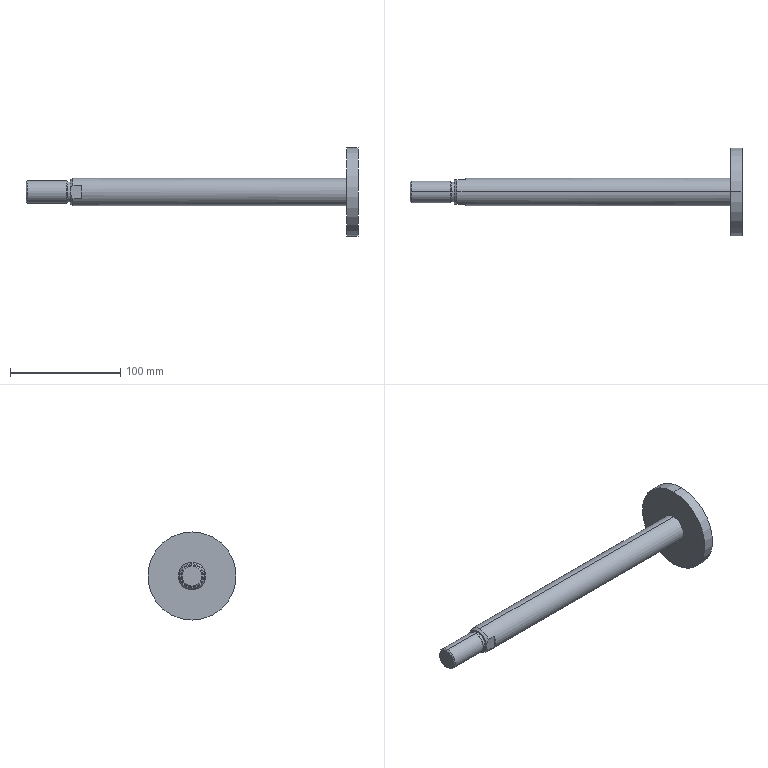Part | SolidWorks | features BaseBody 1 | 1 solid | 24 faces | box 301 x 80 x 80 mm | volume 185506 mm3 | plane 9 | cylinder 8 | cone 7 | commonest cylinder face diameters 18 x2 20 x2 25 x2 80 x2
STEP:
#1=CARTESIAN_POINT('',(205.,0.,12.5));
#2=VERTEX_POINT('',#1);
#3=CARTESIAN_POINT('',(205.,0.,-12.5));
#4=VERTEX_POINT('',#3);
#5=CARTESIAN_POINT('',(205.,0.,0.));
#6=DIRECTION('',(-1.,0.,0.));
#7=DIRECTION('',(0.,0.,1.));
#8=AXIS2_PLACEMENT_3D('',#5,#6,#7);
#9=CIRCLE('',#8,12.5);
#10=EDGE_CURVE('',#2,#4,#9,.T.);
#11=ORIENTED_EDGE('',*,*,#10,.T.);
#12=CARTESIAN_POINT('',(-43.402,0.,-12.5));
#13=VERTEX_POINT('',#12);
#14=CARTESIAN_POINT('',(215.,0.,-12.5));
#15=DIRECTION('',(-1.,0.,0.));
#16=VECTOR('',#15,1000.);
#17=LINE('',#14,#16);
#18=EDGE_CURVE('',#4,#13,#17,.T.);
#19=ORIENTED_EDGE('',*,*,#18,.T.);
#20=CARTESIAN_POINT('',(-43.402,11.,-5.937));
#21=VERTEX_POINT('',#20);
#22=CARTESIAN_POINT('',(-43.402,0.,0.));
#23=DIRECTION('',(1.,0.,0.));
#24=DIRECTION('',(0.,0.,1.));
#25=AXIS2_PLACEMENT_3D('',#22,#23,#24);
#26=CIRCLE('',#25,12.5);
#27=EDGE_CURVE('',#13,#21,#26,.T.);
#28=ORIENTED_EDGE('',*,*,#27,.T.);
#29=CARTESIAN_POINT('',(-36.,11.,-5.937));
#30=VERTEX_POINT('',#29);
#31=CARTESIAN_POINT('',(215.,11.,-5.937));
#32=DIRECTION('',(1.,0.,0.));
#33=VECTOR('',#32,1000.);
#34=LINE('',#31,#33);
#35=EDGE_CURVE('',#21,#30,#34,.T.);
#36=ORIENTED_EDGE('',*,*,#35,.T.);
#37=CARTESIAN_POINT('',(-36.,11.,5.937));
#38=VERTEX_POINT('',#37);
#39=CARTESIAN_POINT('',(-36.,0.,0.));
#40=DIRECTION('',(1.,0.,0.));
#41=DIRECTION('',(0.,0.,1.));
#42=AXIS2_PLACEMENT_3D('',#39,#40,#41);
#43=CIRCLE('',#42,12.5);
#44=EDGE_CURVE('',#30,#38,#43,.T.);
#45=ORIENTED_EDGE('',*,*,#44,.T.);
#46=CARTESIAN_POINT('',(-43.402,11.,5.937));
#47=VERTEX_POINT('',#46);
#48=CARTESIAN_POINT('',(215.,11.,5.937));
#49=DIRECTION('',(-1.,0.,0.));
#50=VECTOR('',#49,1000.);
#51=LINE('',#48,#50);
#52=EDGE_CURVE('',#38,#47,#51,.T.);
#53=ORIENTED_EDGE('',*,*,#52,.T.);
#54=CARTESIAN_POINT('',(-43.402,0.,12.5));
#55=VERTEX_POINT('',#54);
#56=CARTESIAN_POINT('',(-43.402,0.,0.));
#57=DIRECTION('',(1.,0.,0.));
#58=DIRECTION('',(0.,0.,1.));
#59=AXIS2_PLACEMENT_3D('',#56,#57,#58);
#60=CIRCLE('',#59,12.5);
#61=EDGE_CURVE('',#47,#55,#60,.T.);
#62=ORIENTED_EDGE('',*,*,#61,.T.);
#63=CARTESIAN_POINT('',(215.,0.,12.5));
#64=DIRECTION('',(-1.,0.,0.));
#65=VECTOR('',#64,1000.);
#66=LINE('',#63,#65);
#67=EDGE_CURVE('',#2,#55,#66,.T.);
#68=ORIENTED_EDGE('',*,*,#67,.F.);
#69=EDGE_LOOP('',(#11,#19,#28,#36,#45,#53,#62,#68));
#70=FACE_OUTER_BOUND('',#69,.T.);
#71=CARTESIAN_POINT('',(215.,0.,0.));
#72=DIRECTION('',(-1.,0.,0.));
#73=DIRECTION('',(0.,0.,1.));
#74=AXIS2_PLACEMENT_3D('',#71,#72,#73);
#75=CYLINDRICAL_SURFACE('',#74,12.5);
#76=ADVANCED_FACE('',(#70),#75,.T.);
#77=CARTESIAN_POINT('',(-46.,-11.,0.));
#78=VERTEX_POINT('',#77);
#79=CARTESIAN_POINT('',(-46.,0.,-11.));
#80=VERTEX_POINT('',#79);
#81=CARTESIAN_POINT('',(-46.,0.,0.));
#82=DIRECTION('',(1.,0.,0.));
#83=DIRECTION('',(0.,0.,-1.));
#84=AXIS2_PLACEMENT_3D('',#81,#82,#83);
#85=CIRCLE('',#84,11.);
#86=EDGE_CURVE('',#78,#80,#85,.T.);
#87=ORIENTED_EDGE('',*,*,#86,.T.);
#88=CARTESIAN_POINT('',(-43.402,0.,-12.5));
#89=DIRECTION('',(0.866,0.,-0.5));
#90=VECTOR('',#89,1000.);
#91=LINE('',#88,#90);
#92=EDGE_CURVE('',#80,#13,#91,.T.);
#93=ORIENTED_EDGE('',*,*,#92,.T.);
#94=CARTESIAN_POINT('',(-43.402,-11.,-5.937));
#95=VERTEX_POINT('',#94);
#96=CARTESIAN_POINT('',(-43.402,0.,0.));
#97=DIRECTION('',(1.,0.,0.));
#98=DIRECTION('',(0.,0.,1.));
#99=AXIS2_PLACEMENT_3D('',#96,#97,#98);
#100=CIRCLE('',#99,12.5);
#101=EDGE_CURVE('',#95,#13,#100,.T.);
#102=ORIENTED_EDGE('',*,*,#101,.F.);
#103=CARTESIAN_POINT('',(-43.402,-11.,-5.937));
#104=CARTESIAN_POINT('',(-43.753,-11.,-5.51));
#105=CARTESIAN_POINT('',(-44.085,-11.,-5.071));
#106=CARTESIAN_POINT('',(-44.695,-11.,-4.161));
#107=CARTESIAN_POINT('',(-44.973,-11.,-3.69));
#108=CARTESIAN_POINT('',(-45.332,-11.,-2.948));
#109=CARTESIAN_POINT('',(-45.442,-11.,-2.694));
#110=CARTESIAN_POINT('',(-45.637,-11.,-2.173));
#111=CARTESIAN_POINT('',(-45.721,-11.,-1.908));
#112=CARTESIAN_POINT('',(-45.926,-11.,-1.106));
#113=CARTESIAN_POINT('',(-46.,-11.,-0.5595));
#114=CARTESIAN_POINT('',(-46.,-11.,0.));
#115=B_SPLINE_CURVE_WITH_KNOTS('',3,(#103,#104,#105,#106,#107,#108,#109,#110,#111,#112,#113,#114),.UNSPECIFIED.,.F.,.F.,(4,2,2,2,2,4),(0.,0.001642,0.003283,0.004104,0.004925,0.006566),.UNSPECIFIED.);
#116=EDGE_CURVE('',#95,#78,#115,.T.);
#117=ORIENTED_EDGE('',*,*,#116,.T.);
#118=EDGE_LOOP('',(#87,#93,#102,#117));
#119=FACE_OUTER_BOUND('',#118,.T.);
#120=CARTESIAN_POINT('',(-43.402,0.,0.));
#121=DIRECTION('',(1.,0.,0.));
#122=DIRECTION('',(0.,0.,-1.));
#123=AXIS2_PLACEMENT_3D('',#120,#121,#122);
#124=CONICAL_SURFACE('',#123,12.5,0.5236);
#125=ADVANCED_FACE('',(#119),#124,.T.);
#126=CARTESIAN_POINT('',(215.,0.,40.));
#127=VERTEX_POINT('',#126);
#128=CARTESIAN_POINT('',(215.,0.,-40.));
#129=VERTEX_POINT('',#128);
#130=CARTESIAN_POINT('',(215.,0.,0.));
#131=DIRECTION('',(-1.,0.,0.));
#132=DIRECTION('',(0.,0.,1.));
#133=AXIS2_PLACEMENT_3D('',#130,#131,#132);
#134=CIRCLE('',#133,40.);
#135=EDGE_CURVE('',#127,#129,#134,.T.);
#136=ORIENTED_EDGE('',*,*,#135,.T.);
#137=CARTESIAN_POINT('',(205.,0.,-40.));
#138=VERTEX_POINT('',#137);
#139=CARTESIAN_POINT('',(215.,0.,-40.));
#140=DIRECTION('',(-1.,0.,0.));
#141=VECTOR('',#140,1000.);
#142=LINE('',#139,#141);
#143=EDGE_CURVE('',#129,#138,#142,.T.);
#144=ORIENTED_EDGE('',*,*,#143,.T.);
#145=CARTESIAN_POINT('',(205.,0.,40.));
#146=VERTEX_POINT('',#145);
#147=CARTESIAN_POINT('',(205.,0.,0.));
#148=DIRECTION('',(1.,0.,0.));
#149=DIRECTION('',(0.,0.,1.));
#150=AXIS2_PLACEMENT_3D('',#147,#148,#149);
#151=CIRCLE('',#150,40.);
#152=EDGE_CURVE('',#138,#146,#151,.T.);
#153=ORIENTED_EDGE('',*,*,#152,.T.);
#154=CARTESIAN_POINT('',(215.,0.,40.));
#155=DIRECTION('',(-1.,0.,0.));
#156=VECTOR('',#155,1000.);
#157=LINE('',#154,#156);
#158=EDGE_CURVE('',#127,#146,#157,.T.);
#159=ORIENTED_EDGE('',*,*,#158,.F.);
#160=EDGE_LOOP('',(#136,#144,#153,#159));
#161=FACE_OUTER_BOUND('',#160,.T.);
#162=CARTESIAN_POINT('',(215.,0.,0.));
#163=DIRECTION('',(-1.,0.,0.));
#164=DIRECTION('',(0.,0.,1.));
#165=AXIS2_PLACEMENT_3D('',#162,#163,#164);
#166=CYLINDRICAL_SURFACE('',#165,40.);
#167=ADVANCED_FACE('',(#161),#166,.T.);
#168=CARTESIAN_POINT('',(-46.,0.,9.));
#169=VERTEX_POINT('',#168);
#170=CARTESIAN_POINT('',(-46.,0.,-9.));
#171=VERTEX_POINT('',#170);
#172=CARTESIAN_POINT('',(-46.,0.,0.));
#173=DIRECTION('',(-1.,0.,0.));
#174=DIRECTION('',(0.,0.,1.));
#175=AXIS2_PLACEMENT_3D('',#172,#173,#174);
#176=CIRCLE('',#175,9.);
#177=EDGE_CURVE('',#169,#171,#176,.T.);
#178=ORIENTED_EDGE('',*,*,#177,.T.);
#179=CARTESIAN_POINT('',(-48.25,0.,-9.));
#180=VERTEX_POINT('',#179);
#181=CARTESIAN_POINT('',(215.,0.,-9.));
#182=DIRECTION('',(-1.,0.,0.));
#183=VECTOR('',#182,1000.);
#184=LINE('',#181,#183);
#185=EDGE_CURVE('',#171,#180,#184,.T.);
#186=ORIENTED_EDGE('',*,*,#185,.T.);
#187=CARTESIAN_POINT('',(-48.25,0.,9.));
#188=VERTEX_POINT('',#187);
#189=CARTESIAN_POINT('',(-48.25,0.,0.));
#190=DIRECTION('',(1.,0.,0.));
#191=DIRECTION('',(0.,0.,1.));
#192=AXIS2_PLACEMENT_3D('',#189,#190,#191);
#193=CIRCLE('',#192,9.);
#194=EDGE_CURVE('',#180,#188,#193,.T.);
#195=ORIENTED_EDGE('',*,*,#194,.T.);
#196=CARTESIAN_POINT('',(215.,0.,9.));
#197=DIRECTION('',(-1.,0.,0.));
#198=VECTOR('',#197,1000.);
#199=LINE('',#196,#198);
#200=EDGE_CURVE('',#169,#188,#199,.T.);
#201=ORIENTED_EDGE('',*,*,#200,.F.);
#202=EDGE_LOOP('',(#178,#186,#195,#201));
#203=FACE_OUTER_BOUND('',#202,.T.);
#204=CARTESIAN_POINT('',(215.,0.,0.));
#205=DIRECTION('',(-1.,0.,0.));
#206=DIRECTION('',(0.,0.,1.));
#207=AXIS2_PLACEMENT_3D('',#204,#205,#206);
#208=CYLINDRICAL_SURFACE('',#207,9.);
#209=ADVANCED_FACE('',(#203),#208,.T.);
#210=CARTESIAN_POINT('',(-48.25,0.,9.08));
#211=VERTEX_POINT('',#210);
#212=CARTESIAN_POINT('',(-48.25,0.,-9.08));
#213=VERTEX_POINT('',#212);
#214=CARTESIAN_POINT('',(-48.25,0.,0.));
#215=DIRECTION('',(-1.,0.,0.));
#216=DIRECTION('',(0.,0.,1.));
#217=AXIS2_PLACEMENT_3D('',#214,#215,#216);
#218=CIRCLE('',#217,9.08);
#219=EDGE_CURVE('',#211,#213,#218,.T.);
#220=ORIENTED_EDGE('',*,*,#219,.T.);
#221=CARTESIAN_POINT('',(-49.17,0.,-10.));
#222=VERTEX_POINT('',#221);
#223=CARTESIAN_POINT('',(-49.17,0.,-10.));
#224=DIRECTION('',(-0.7071,0.,-0.7071));
#225=VECTOR('',#224,1000.);
#226=LINE('',#223,#225);
#227=EDGE_CURVE('',#213,#222,#226,.T.);
#228=ORIENTED_EDGE('',*,*,#227,.T.);
#229=CARTESIAN_POINT('',(-49.17,0.,10.));
#230=VERTEX_POINT('',#229);
#231=CARTESIAN_POINT('',(-49.17,0.,0.));
#232=DIRECTION('',(1.,0.,0.));
#233=DIRECTION('',(0.,0.,1.));
#234=AXIS2_PLACEMENT_3D('',#231,#232,#233);
#235=CIRCLE('',#234,10.);
#236=EDGE_CURVE('',#222,#230,#235,.T.);
#237=ORIENTED_EDGE('',*,*,#236,.T.);
#238=CARTESIAN_POINT('',(-49.17,0.,10.));
#239=DIRECTION('',(-0.7071,0.,0.7071));
#240=VECTOR('',#239,1000.);
#241=LINE('',#238,#240);
#242=EDGE_CURVE('',#211,#230,#241,.T.);
#243=ORIENTED_EDGE('',*,*,#242,.F.);
#244=EDGE_LOOP('',(#220,#228,#237,#243));
#245=FACE_OUTER_BOUND('',#244,.T.);
#246=CARTESIAN_POINT('',(-49.17,0.,0.));
#247=DIRECTION('',(-1.,0.,0.));
#248=DIRECTION('',(0.,0.,1.));
#249=AXIS2_PLACEMENT_3D('',#246,#247,#248);
#250=CONICAL_SURFACE('',#249,10.,0.7854);
#251=ADVANCED_FACE('',(#245),#250,.T.);
#252=ORIENTED_EDGE('',*,*,#236,.F.);
#253=CARTESIAN_POINT('',(-85.08,0.,-10.));
#254=VERTEX_POINT('',#253);
#255=CARTESIAN_POINT('',(215.,0.,-10.));
#256=DIRECTION('',(-1.,0.,0.));
#257=VECTOR('',#256,1000.);
#258=LINE('',#255,#257);
#259=EDGE_CURVE('',#222,#254,#258,.T.);
#260=ORIENTED_EDGE('',*,*,#259,.T.);
#261=CARTESIAN_POINT('',(-85.08,0.,10.));
#262=VERTEX_POINT('',#261);
#263=CARTESIAN_POINT('',(-85.08,0.,0.));
#264=DIRECTION('',(1.,0.,0.));
#265=DIRECTION('',(0.,0.,1.));
#266=AXIS2_PLACEMENT_3D('',#263,#264,#265);
#267=CIRCLE('',#266,10.);
#268=EDGE_CURVE('',#254,#262,#267,.T.);
#269=ORIENTED_EDGE('',*,*,#268,.T.);
#270=CARTESIAN_POINT('',(215.,0.,10.));
#271=DIRECTION('',(-1.,0.,0.));
#272=VECTOR('',#271,1000.);
#273=LINE('',#270,#272);
#274=EDGE_CURVE('',#230,#262,#273,.T.);
#275=ORIENTED_EDGE('',*,*,#274,.F.);
#276=EDGE_LOOP('',(#252,#260,#269,#275));
#277=FACE_OUTER_BOUND('',#276,.T.);
#278=CARTESIAN_POINT('',(215.,0.,0.));
#279=DIRECTION('',(-1.,0.,0.));
#280=DIRECTION('',(0.,0.,1.));
#281=AXIS2_PLACEMENT_3D('',#278,#279,#280);
#282=CYLINDRICAL_SURFACE('',#281,10.);
#283=ADVANCED_FACE('',(#277),#282,.T.);
#284=CARTESIAN_POINT('',(-86.,0.,-9.08));
#285=VERTEX_POINT('',#284);
#286=CARTESIAN_POINT('',(-86.,0.,9.08));
#287=VERTEX_POINT('',#286);
#288=CARTESIAN_POINT('',(-86.,0.,0.));
#289=DIRECTION('',(1.,0.,0.));
#290=DIRECTION('',(0.,0.,-1.));
#291=AXIS2_PLACEMENT_3D('',#288,#289,#290);
#292=CIRCLE('',#291,9.08);
#293=EDGE_CURVE('',#285,#287,#292,.T.);
#294=ORIENTED_EDGE('',*,*,#293,.T.);
#295=CARTESIAN_POINT('',(-85.08,0.,10.));
#296=DIRECTION('',(0.7071,0.,0.7071));
#297=VECTOR('',#296,1000.);
#298=LINE('',#295,#297);
#299=EDGE_CURVE('',#287,#262,#298,.T.);
#300=ORIENTED_EDGE('',*,*,#299,.T.);
#301=ORIENTED_EDGE('',*,*,#268,.F.);
#302=CARTESIAN_POINT('',(-85.08,0.,-10.));
#303=DIRECTION('',(0.7071,0.,-0.7071));
#304=VECTOR('',#303,1000.);
#305=LINE('',#302,#304);
#306=EDGE_CURVE('',#285,#254,#305,.T.);
#307=ORIENTED_EDGE('',*,*,#306,.F.);
#308=EDGE_LOOP('',(#294,#300,#301,#307));
#309=FACE_OUTER_BOUND('',#308,.T.);
#310=CARTESIAN_POINT('',(-85.08,0.,0.));
#311=DIRECTION('',(1.,0.,0.));
#312=DIRECTION('',(0.,0.,-1.));
#313=AXIS2_PLACEMENT_3D('',#310,#311,#312);
#314=CONICAL_SURFACE('',#313,10.,0.7854);
#315=ADVANCED_FACE('',(#309),#314,.T.);
#316=ORIENTED_EDGE('',*,*,#18,.F.);
#317=CARTESIAN_POINT('',(205.,0.,0.));
#318=DIRECTION('',(-1.,0.,0.));
#319=DIRECTION('',(0.,0.,1.));
#320=AXIS2_PLACEMENT_3D('',#317,#318,#319);
#321=CIRCLE('',#320,12.5);
#322=EDGE_CURVE('',#4,#2,#321,.T.);
#323=ORIENTED_EDGE('',*,*,#322,.T.);
#324=ORIENTED_EDGE('',*,*,#67,.T.);
#325=CARTESIAN_POINT('',(-43.402,-11.,5.937));
#326=VERTEX_POINT('',#325);
#327=CARTESIAN_POINT('',(-43.402,0.,0.));
#328=DIRECTION('',(1.,0.,0.));
#329=DIRECTION('',(0.,0.,1.));
#330=AXIS2_PLACEMENT_3D('',#327,#328,#329);
#331=CIRCLE('',#330,12.5);
#332=EDGE_CURVE('',#55,#326,#331,.T.);
#333=ORIENTED_EDGE('',*,*,#332,.T.);
#334=CARTESIAN_POINT('',(-36.,-11.,5.937));
#335=VERTEX_POINT('',#334);
#336=CARTESIAN_POINT('',(215.,-11.,5.937));
#337=DIRECTION('',(1.,0.,0.));
#338=VECTOR('',#337,1000.);
#339=LINE('',#336,#338);
#340=EDGE_CURVE('',#326,#335,#339,.T.);
#341=ORIENTED_EDGE('',*,*,#340,.T.);
#342=CARTESIAN_POINT('',(-36.,-11.,-5.937));
#343=VERTEX_POINT('',#342);
#344=CARTESIAN_POINT('',(-36.,0.,0.));
#345=DIRECTION('',(1.,0.,0.));
#346=DIRECTION('',(0.,0.,1.));
#347=AXIS2_PLACEMENT_3D('',#344,#345,#346);
#348=CIRCLE('',#347,12.5);
#349=EDGE_CURVE('',#335,#343,#348,.T.);
#350=ORIENTED_EDGE('',*,*,#349,.T.);
#351=CARTESIAN_POINT('',(215.,-11.,-5.937));
#352=DIRECTION('',(-1.,0.,0.));
#353=VECTOR('',#352,1000.);
#354=LINE('',#351,#353);
#355=EDGE_CURVE('',#343,#95,#354,.T.);
#356=ORIENTED_EDGE('',*,*,#355,.T.);
#357=ORIENTED_EDGE('',*,*,#101,.T.);
#358=EDGE_LOOP('',(#316,#323,#324,#333,#341,#350,#356,#357));
#359=FACE_OUTER_BOUND('',#358,.T.);
#360=CARTESIAN_POINT('',(215.,0.,0.));
#361=DIRECTION('',(-1.,0.,0.));
#362=DIRECTION('',(0.,0.,1.));
#363=AXIS2_PLACEMENT_3D('',#360,#361,#362);
#364=CYLINDRICAL_SURFACE('',#363,12.5);
#365=ADVANCED_FACE('',(#359),#364,.T.);
#366=ORIENTED_EDGE('',*,*,#61,.F.);
#367=CARTESIAN_POINT('',(-46.,11.,0.));
#368=VERTEX_POINT('',#367);
#369=CARTESIAN_POINT('',(-43.402,11.,5.937));
#370=CARTESIAN_POINT('',(-43.753,11.,5.51));
#371=CARTESIAN_POINT('',(-44.085,11.,5.071));
#372=CARTESIAN_POINT('',(-44.695,11.,4.161));
#373=CARTESIAN_POINT('',(-44.973,11.,3.69));
#374=CARTESIAN_POINT('',(-45.332,11.,2.948));
#375=CARTESIAN_POINT('',(-45.442,11.,2.694));
#376=CARTESIAN_POINT('',(-45.637,11.,2.173));
#377=CARTESIAN_POINT('',(-45.721,11.,1.908));
#378=CARTESIAN_POINT('',(-45.926,11.,1.106));
#379=CARTESIAN_POINT('',(-46.,11.,0.5595));
#380=CARTESIAN_POINT('',(-46.,11.,0.));
#381=B_SPLINE_CURVE_WITH_KNOTS('',3,(#369,#370,#371,#372,#373,#374,#375,#376,#377,#378,#379,#380),.UNSPECIFIED.,.F.,.F.,(4,2,2,2,2,4),(0.,0.001642,0.003283,0.004104,0.004925,0.006566),.UNSPECIFIED.);
#382=EDGE_CURVE('',#47,#368,#381,.T.);
#383=ORIENTED_EDGE('',*,*,#382,.T.);
#384=CARTESIAN_POINT('',(-46.,0.,0.));
#385=DIRECTION('',(1.,0.,0.));
#386=DIRECTION('',(0.,0.,-1.));
#387=AXIS2_PLACEMENT_3D('',#384,#385,#386);
#388=CIRCLE('',#387,11.);
#389=EDGE_CURVE('',#368,#78,#388,.T.);
#390=ORIENTED_EDGE('',*,*,#389,.T.);
#391=CARTESIAN_POINT('',(-46.,-11.,0.));
#392=CARTESIAN_POINT('',(-46.,-11.,0.5593));
#393=CARTESIAN_POINT('',(-45.926,-11.,1.104));
#394=CARTESIAN_POINT('',(-45.654,-11.,2.169));
#395=CARTESIAN_POINT('',(-45.454,-11.,2.694));
#396=CARTESIAN_POINT('',(-44.975,-11.,3.687));
#397=CARTESIAN_POINT('',(-44.696,-11.,4.159));
#398=CARTESIAN_POINT('',(-44.086,-11.,5.071));
#399=CARTESIAN_POINT('',(-43.753,-11.,5.51));
#400=CARTESIAN_POINT('',(-43.402,-11.,5.937));
#401=B_SPLINE_CURVE_WITH_KNOTS('',3,(#391,#392,#393,#394,#395,#396,#397,#398,#399,#400),.UNSPECIFIED.,.F.,.F.,(4,2,2,2,4),(0.,0.001646,0.003293,0.004939,0.006586),.UNSPECIFIED.);
#402=EDGE_CURVE('',#78,#326,#401,.T.);
#403=ORIENTED_EDGE('',*,*,#402,.T.);
#404=ORIENTED_EDGE('',*,*,#332,.F.);
#405=EDGE_LOOP('',(#366,#383,#390,#403,#404));
#406=FACE_OUTER_BOUND('',#405,.T.);
#407=CARTESIAN_POINT('',(-43.402,0.,0.));
#408=DIRECTION('',(1.,0.,0.));
#409=DIRECTION('',(0.,0.,-1.));
#410=AXIS2_PLACEMENT_3D('',#407,#408,#409);
#411=CONICAL_SURFACE('',#410,12.5,0.5236);
#412=ADVANCED_FACE('',(#406),#411,.T.);
#413=ORIENTED_EDGE('',*,*,#35,.F.);
#414=CARTESIAN_POINT('',(-46.,11.,0.));
#415=CARTESIAN_POINT('',(-46.,11.,-0.5593));
#416=CARTESIAN_POINT('',(-45.926,11.,-1.104));
#417=CARTESIAN_POINT('',(-45.654,11.,-2.169));
#418=CARTESIAN_POINT('',(-45.454,11.,-2.694));
#419=CARTESIAN_POINT('',(-44.975,11.,-3.687));
#420=CARTESIAN_POINT('',(-44.696,11.,-4.159));
#421=CARTESIAN_POINT('',(-44.086,11.,-5.071));
#422=CARTESIAN_POINT('',(-43.753,11.,-5.51));
#423=CARTESIAN_POINT('',(-43.402,11.,-5.937));
#424=B_SPLINE_CURVE_WITH_KNOTS('',3,(#414,#415,#416,#417,#418,#419,#420,#421,#422,#423),.UNSPECIFIED.,.F.,.F.,(4,2,2,2,4),(0.,0.001646,0.003293,0.004939,0.006586),.UNSPECIFIED.);
#425=EDGE_CURVE('',#368,#21,#424,.T.);
#426=ORIENTED_EDGE('',*,*,#425,.F.);
#427=ORIENTED_EDGE('',*,*,#382,.F.);
#428=ORIENTED_EDGE('',*,*,#52,.F.);
#429=CARTESIAN_POINT('',(-36.,11.,-14.5));
#430=DIRECTION('',(0.,0.,1.));
#431=VECTOR('',#430,1000.);
#432=LINE('',#429,#431);
#433=EDGE_CURVE('',#30,#38,#432,.T.);
#434=ORIENTED_EDGE('',*,*,#433,.F.);
#435=EDGE_LOOP('',(#413,#426,#427,#428,#434));
#436=FACE_OUTER_BOUND('',#435,.T.);
#437=CARTESIAN_POINT('',(-36.,11.,-14.5));
#438=DIRECTION('',(0.,-1.,0.));
#439=DIRECTION('',(0.,0.,-1.));
#440=AXIS2_PLACEMENT_3D('',#437,#438,#439);
#441=PLANE('',#440);
#442=ADVANCED_FACE('',(#436),#441,.F.);
#443=ORIENTED_EDGE('',*,*,#44,.F.);
#444=ORIENTED_EDGE('',*,*,#433,.T.);
#445=EDGE_LOOP('',(#443,#444));
#446=FACE_OUTER_BOUND('',#445,.T.);
#447=CARTESIAN_POINT('',(-36.,0.,0.));
#448=DIRECTION('',(1.,0.,0.));
#449=DIRECTION('',(0.,0.,-1.));
#450=AXIS2_PLACEMENT_3D('',#447,#448,#449);
#451=PLANE('',#450);
#452=ADVANCED_FACE('',(#446),#451,.F.);
#453=ORIENTED_EDGE('',*,*,#92,.F.);
#454=CARTESIAN_POINT('',(-46.,0.,0.));
#455=DIRECTION('',(1.,0.,0.));
#456=DIRECTION('',(0.,0.,-1.));
#457=AXIS2_PLACEMENT_3D('',#454,#455,#456);
#458=CIRCLE('',#457,11.);
#459=EDGE_CURVE('',#80,#368,#458,.T.);
#460=ORIENTED_EDGE('',*,*,#459,.T.);
#461=ORIENTED_EDGE('',*,*,#425,.T.);
#462=ORIENTED_EDGE('',*,*,#27,.F.);
#463=EDGE_LOOP('',(#453,#460,#461,#462));
#464=FACE_OUTER_BOUND('',#463,.T.);
#465=CARTESIAN_POINT('',(-43.402,0.,0.));
#466=DIRECTION('',(1.,0.,0.));
#467=DIRECTION('',(0.,0.,-1.));
#468=AXIS2_PLACEMENT_3D('',#465,#466,#467);
#469=CONICAL_SURFACE('',#468,12.5,0.5236);
#470=ADVANCED_FACE('',(#464),#469,.T.);
#471=CARTESIAN_POINT('',(205.,0.,0.));
#472=DIRECTION('',(1.,0.,0.));
#473=DIRECTION('',(0.,0.,1.));
#474=AXIS2_PLACEMENT_3D('',#471,#472,#473);
#475=CIRCLE('',#474,40.);
#476=EDGE_CURVE('',#146,#138,#475,.T.);
#477=ORIENTED_EDGE('',*,*,#476,.F.);
#478=ORIENTED_EDGE('',*,*,#152,.F.);
#479=EDGE_LOOP('',(#477,#478));
#480=FACE_OUTER_BOUND('',#479,.T.);
#481=ORIENTED_EDGE('',*,*,#10,.F.);
#482=ORIENTED_EDGE('',*,*,#322,.F.);
#483=EDGE_LOOP('',(#481,#482));
#484=FACE_BOUND('',#483,.T.);
#485=CARTESIAN_POINT('',(205.,12.5,0.));
#486=DIRECTION('',(1.,0.,0.));
#487=DIRECTION('',(0.,0.,-1.));
#488=AXIS2_PLACEMENT_3D('',#485,#486,#487);
#489=PLANE('',#488);
#490=ADVANCED_FACE('',(#480,#484),#489,.F.);
#491=ORIENTED_EDGE('',*,*,#340,.F.);
#492=ORIENTED_EDGE('',*,*,#402,.F.);
#493=ORIENTED_EDGE('',*,*,#116,.F.);
#494=ORIENTED_EDGE('',*,*,#355,.F.);
#495=CARTESIAN_POINT('',(-36.,-11.,14.5));
#496=DIRECTION('',(0.,0.,-1.));
#497=VECTOR('',#496,1000.);
#498=LINE('',#495,#497);
#499=EDGE_CURVE('',#335,#343,#498,.T.);
#500=ORIENTED_EDGE('',*,*,#499,.F.);
#501=EDGE_LOOP('',(#491,#492,#493,#494,#500));
#502=FACE_OUTER_BOUND('',#501,.T.);
#503=CARTESIAN_POINT('',(-36.,-11.,14.5));
#504=DIRECTION('',(0.,1.,0.));
#505=DIRECTION('',(0.,0.,1.));
#506=AXIS2_PLACEMENT_3D('',#503,#504,#505);
#507=PLANE('',#506);
#508=ADVANCED_FACE('',(#502),#507,.F.);
#509=ORIENTED_EDGE('',*,*,#349,.F.);
#510=ORIENTED_EDGE('',*,*,#499,.T.);
#511=EDGE_LOOP('',(#509,#510));
#512=FACE_OUTER_BOUND('',#511,.T.);
#513=CARTESIAN_POINT('',(-36.,0.,0.));
#514=DIRECTION('',(1.,0.,0.));
#515=DIRECTION('',(0.,0.,-1.));
#516=AXIS2_PLACEMENT_3D('',#513,#514,#515);
#517=PLANE('',#516);
#518=ADVANCED_FACE('',(#512),#517,.F.);
#519=ORIENTED_EDGE('',*,*,#86,.F.);
#520=ORIENTED_EDGE('',*,*,#389,.F.);
#521=ORIENTED_EDGE('',*,*,#459,.F.);
#522=EDGE_LOOP('',(#519,#520,#521));
#523=FACE_OUTER_BOUND('',#522,.T.);
#524=ORIENTED_EDGE('',*,*,#177,.F.);
#525=CARTESIAN_POINT('',(-46.,0.,0.));
#526=DIRECTION('',(-1.,0.,0.));
#527=DIRECTION('',(0.,0.,1.));
#528=AXIS2_PLACEMENT_3D('',#525,#526,#527);
#529=CIRCLE('',#528,9.);
#530=EDGE_CURVE('',#171,#169,#529,.T.);
#531=ORIENTED_EDGE('',*,*,#530,.F.);
#532=EDGE_LOOP('',(#524,#531));
#533=FACE_BOUND('',#532,.T.);
#534=CARTESIAN_POINT('',(-46.,9.,0.));
#535=DIRECTION('',(1.,0.,0.));
#536=DIRECTION('',(0.,0.,-1.));
#537=AXIS2_PLACEMENT_3D('',#534,#535,#536);
#538=PLANE('',#537);
#539=ADVANCED_FACE('',(#523,#533),#538,.F.);
#540=ORIENTED_EDGE('',*,*,#143,.F.);
#541=CARTESIAN_POINT('',(215.,0.,0.));
#542=DIRECTION('',(-1.,0.,0.));
#543=DIRECTION('',(0.,0.,1.));
#544=AXIS2_PLACEMENT_3D('',#541,#542,#543);
#545=CIRCLE('',#544,40.);
#546=EDGE_CURVE('',#129,#127,#545,.T.);
#547=ORIENTED_EDGE('',*,*,#546,.T.);
#548=ORIENTED_EDGE('',*,*,#158,.T.);
#549=ORIENTED_EDGE('',*,*,#476,.T.);
#550=EDGE_LOOP('',(#540,#547,#548,#549));
#551=FACE_OUTER_BOUND('',#550,.T.);
#552=CARTESIAN_POINT('',(215.,0.,0.));
#553=DIRECTION('',(-1.,0.,0.));
#554=DIRECTION('',(0.,0.,1.));
#555=AXIS2_PLACEMENT_3D('',#552,#553,#554);
#556=CYLINDRICAL_SURFACE('',#555,40.);
#557=ADVANCED_FACE('',(#551),#556,.T.);
#558=ORIENTED_EDGE('',*,*,#185,.F.);
#559=ORIENTED_EDGE('',*,*,#530,.T.);
#560=ORIENTED_EDGE('',*,*,#200,.T.);
#561=CARTESIAN_POINT('',(-48.25,0.,0.));
#562=DIRECTION('',(1.,0.,0.));
#563=DIRECTION('',(0.,0.,1.));
#564=AXIS2_PLACEMENT_3D('',#561,#562,#563);
#565=CIRCLE('',#564,9.);
#566=EDGE_CURVE('',#188,#180,#565,.T.);
#567=ORIENTED_EDGE('',*,*,#566,.T.);
#568=EDGE_LOOP('',(#558,#559,#560,#567));
#569=FACE_OUTER_BOUND('',#568,.T.);
#570=CARTESIAN_POINT('',(215.,0.,0.));
#571=DIRECTION('',(-1.,0.,0.));
#572=DIRECTION('',(0.,0.,1.));
#573=AXIS2_PLACEMENT_3D('',#570,#571,#572);
#574=CYLINDRICAL_SURFACE('',#573,9.);
#575=ADVANCED_FACE('',(#569),#574,.T.);
#576=ORIENTED_EDGE('',*,*,#135,.F.);
#577=ORIENTED_EDGE('',*,*,#546,.F.);
#578=EDGE_LOOP('',(#576,#577));
#579=FACE_OUTER_BOUND('',#578,.T.);
#580=CARTESIAN_POINT('',(215.,40.,0.));
#581=DIRECTION('',(-1.,0.,0.));
#582=DIRECTION('',(0.,0.,1.));
#583=AXIS2_PLACEMENT_3D('',#580,#581,#582);
#584=PLANE('',#583);
#585=ADVANCED_FACE('',(#579),#584,.F.);
#586=ORIENTED_EDGE('',*,*,#566,.F.);
#587=ORIENTED_EDGE('',*,*,#194,.F.);
#588=EDGE_LOOP('',(#586,#587));
#589=FACE_BOUND('',#588,.T.);
#590=ORIENTED_EDGE('',*,*,#219,.F.);
#591=CARTESIAN_POINT('',(-48.25,0.,0.));
#592=DIRECTION('',(-1.,0.,0.));
#593=DIRECTION('',(0.,0.,1.));
#594=AXIS2_PLACEMENT_3D('',#591,#592,#593);
#595=CIRCLE('',#594,9.08);
#596=EDGE_CURVE('',#213,#211,#595,.T.);
#597=ORIENTED_EDGE('',*,*,#596,.F.);
#598=EDGE_LOOP('',(#590,#597));
#599=FACE_OUTER_BOUND('',#598,.T.);
#600=CARTESIAN_POINT('',(-48.25,9.08,0.));
#601=DIRECTION('',(-1.,0.,0.));
#602=DIRECTION('',(0.,0.,1.));
#603=AXIS2_PLACEMENT_3D('',#600,#601,#602);
#604=PLANE('',#603);
#605=ADVANCED_FACE('',(#589,#599),#604,.F.);
#606=ORIENTED_EDGE('',*,*,#227,.F.);
#607=ORIENTED_EDGE('',*,*,#596,.T.);
#608=ORIENTED_EDGE('',*,*,#242,.T.);
#609=CARTESIAN_POINT('',(-49.17,0.,0.));
#610=DIRECTION('',(1.,0.,0.));
#611=DIRECTION('',(0.,0.,1.));
#612=AXIS2_PLACEMENT_3D('',#609,#610,#611);
#613=CIRCLE('',#612,10.);
#614=EDGE_CURVE('',#230,#222,#613,.T.);
#615=ORIENTED_EDGE('',*,*,#614,.T.);
#616=EDGE_LOOP('',(#606,#607,#608,#615));
#617=FACE_OUTER_BOUND('',#616,.T.);
#618=CARTESIAN_POINT('',(-49.17,0.,0.));
#619=DIRECTION('',(-1.,0.,0.));
#620=DIRECTION('',(0.,0.,1.));
#621=AXIS2_PLACEMENT_3D('',#618,#619,#620);
#622=CONICAL_SURFACE('',#621,10.,0.7854);
#623=ADVANCED_FACE('',(#617),#622,.T.);
#624=ORIENTED_EDGE('',*,*,#259,.F.);
#625=ORIENTED_EDGE('',*,*,#614,.F.);
#626=ORIENTED_EDGE('',*,*,#274,.T.);
#627=CARTESIAN_POINT('',(-85.08,0.,0.));
#628=DIRECTION('',(1.,0.,0.));
#629=DIRECTION('',(0.,0.,1.));
#630=AXIS2_PLACEMENT_3D('',#627,#628,#629);
#631=CIRCLE('',#630,10.);
#632=EDGE_CURVE('',#262,#254,#631,.T.);
#633=ORIENTED_EDGE('',*,*,#632,.T.);
#634=EDGE_LOOP('',(#624,#625,#626,#633));
#635=FACE_OUTER_BOUND('',#634,.T.);
#636=CARTESIAN_POINT('',(215.,0.,0.));
#637=DIRECTION('',(-1.,0.,0.));
#638=DIRECTION('',(0.,0.,1.));
#639=AXIS2_PLACEMENT_3D('',#636,#637,#638);
#640=CYLINDRICAL_SURFACE('',#639,10.);
#641=ADVANCED_FACE('',(#635),#640,.T.);
#642=ORIENTED_EDGE('',*,*,#299,.F.);
#643=CARTESIAN_POINT('',(-86.,0.,0.));
#644=DIRECTION('',(1.,0.,0.));
#645=DIRECTION('',(0.,0.,-1.));
#646=AXIS2_PLACEMENT_3D('',#643,#644,#645);
#647=CIRCLE('',#646,9.08);
#648=EDGE_CURVE('',#287,#285,#647,.T.);
#649=ORIENTED_EDGE('',*,*,#648,.T.);
#650=ORIENTED_EDGE('',*,*,#306,.T.);
#651=ORIENTED_EDGE('',*,*,#632,.F.);
#652=EDGE_LOOP('',(#642,#649,#650,#651));
#653=FACE_OUTER_BOUND('',#652,.T.);
#654=CARTESIAN_POINT('',(-85.08,0.,0.));
#655=DIRECTION('',(1.,0.,0.));
#656=DIRECTION('',(0.,0.,-1.));
#657=AXIS2_PLACEMENT_3D('',#654,#655,#656);
#658=CONICAL_SURFACE('',#657,10.,0.7854);
#659=ADVANCED_FACE('',(#653),#658,.T.);
#660=ORIENTED_EDGE('',*,*,#293,.F.);
#661=ORIENTED_EDGE('',*,*,#648,.F.);
#662=EDGE_LOOP('',(#660,#661));
#663=FACE_OUTER_BOUND('',#662,.T.);
#664=CARTESIAN_POINT('',(-86.,0.,0.));
#665=DIRECTION('',(1.,0.,0.));
#666=DIRECTION('',(0.,0.,-1.));
#667=AXIS2_PLACEMENT_3D('',#664,#665,#666);
#668=PLANE('',#667);
#669=ADVANCED_FACE('',(#663),#668,.F.);
#670=CLOSED_SHELL('',(#76,#125,#167,#209,#251,#283,#315,#365,#412,#442,#452,#470,#490,#508,#518,#539,#557,#575,#585,#605,#623,#641,#659,#669));
#671=MANIFOLD_SOLID_BREP('',#670);
#672=CARTESIAN_POINT('',(0.,0.,0.));
#673=DIRECTION('',(0.,0.,1.));
#674=DIRECTION('',(1.,0.,0.));
#675=AXIS2_PLACEMENT_3D('',#672,#673,#674);
#676=(LENGTH_UNIT()NAMED_UNIT(*)SI_UNIT(.MILLI.,.METRE.));
#677=UNCERTAINTY_MEASURE_WITH_UNIT(LENGTH_MEASURE(0.00001),#676,'','');
#678=(NAMED_UNIT(*)PLANE_ANGLE_UNIT()SI_UNIT($,.RADIAN.));
#679=(NAMED_UNIT(*)SI_UNIT($,.STERADIAN.)SOLID_ANGLE_UNIT());
#680=(GEOMETRIC_REPRESENTATION_CONTEXT(3)GLOBAL_UNCERTAINTY_ASSIGNED_CONTEXT((#677))GLOBAL_UNIT_ASSIGNED_CONTEXT((#676,#678,#679))REPRESENTATION_CONTEXT('',''));
#681=ADVANCED_BREP_SHAPE_REPRESENTATION('',(#671,#675),#680);